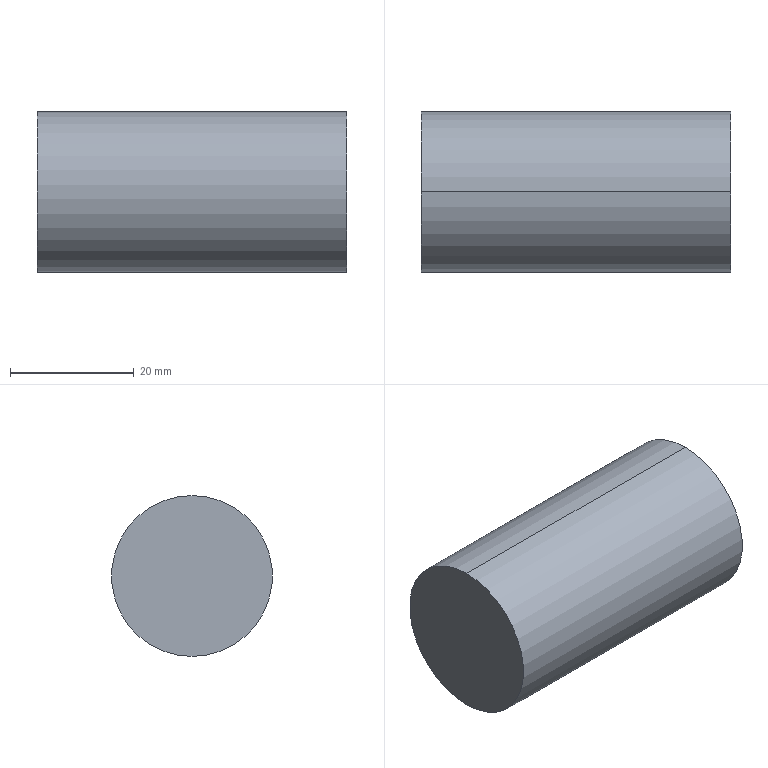Part | SolidWorks | features BaseBody 1 | 1 solid | 4 faces | box 50 x 26.001 x 26.001 mm | volume 26548 mm3 | cylinder 2 | plane 2 | commonest cylinder face diameters 26.001 x2
STEP:
#1=CARTESIAN_POINT('',(-51.,215.,-375.));
#2=VERTEX_POINT('',#1);
#3=CARTESIAN_POINT('',(-51.,215.,-401.));
#4=VERTEX_POINT('',#3);
#5=CARTESIAN_POINT('',(-51.,215.,-388.));
#6=DIRECTION('',(-1.,0.,0.));
#7=DIRECTION('',(0.,0.,1.));
#8=AXIS2_PLACEMENT_3D('',#5,#6,#7);
#9=CIRCLE('',#8,13.);
#10=EDGE_CURVE('',#2,#4,#9,.T.);
#11=ORIENTED_EDGE('',*,*,#10,.T.);
#12=CARTESIAN_POINT('',(-101.,215.,-401.));
#13=VERTEX_POINT('',#12);
#14=CARTESIAN_POINT('',(-51.,215.,-401.));
#15=DIRECTION('',(-1.,0.,0.));
#16=VECTOR('',#15,1000.);
#17=LINE('',#14,#16);
#18=EDGE_CURVE('',#4,#13,#17,.T.);
#19=ORIENTED_EDGE('',*,*,#18,.T.);
#20=CARTESIAN_POINT('',(-101.,215.,-375.));
#21=VERTEX_POINT('',#20);
#22=CARTESIAN_POINT('',(-101.,215.,-388.));
#23=DIRECTION('',(1.,0.,0.));
#24=DIRECTION('',(0.,0.,1.));
#25=AXIS2_PLACEMENT_3D('',#22,#23,#24);
#26=CIRCLE('',#25,13.);
#27=EDGE_CURVE('',#13,#21,#26,.T.);
#28=ORIENTED_EDGE('',*,*,#27,.T.);
#29=CARTESIAN_POINT('',(-51.,215.,-375.));
#30=DIRECTION('',(-1.,0.,0.));
#31=VECTOR('',#30,1000.);
#32=LINE('',#29,#31);
#33=EDGE_CURVE('',#2,#21,#32,.T.);
#34=ORIENTED_EDGE('',*,*,#33,.F.);
#35=EDGE_LOOP('',(#11,#19,#28,#34));
#36=FACE_OUTER_BOUND('',#35,.T.);
#37=CARTESIAN_POINT('',(-51.,215.,-388.));
#38=DIRECTION('',(-1.,0.,0.));
#39=DIRECTION('',(0.,0.,1.));
#40=AXIS2_PLACEMENT_3D('',#37,#38,#39);
#41=CYLINDRICAL_SURFACE('',#40,13.);
#42=ADVANCED_FACE('',(#36),#41,.T.);
#43=ORIENTED_EDGE('',*,*,#18,.F.);
#44=CARTESIAN_POINT('',(-51.,215.,-388.));
#45=DIRECTION('',(-1.,0.,0.));
#46=DIRECTION('',(0.,0.,1.));
#47=AXIS2_PLACEMENT_3D('',#44,#45,#46);
#48=CIRCLE('',#47,13.);
#49=EDGE_CURVE('',#4,#2,#48,.T.);
#50=ORIENTED_EDGE('',*,*,#49,.T.);
#51=ORIENTED_EDGE('',*,*,#33,.T.);
#52=CARTESIAN_POINT('',(-101.,215.,-388.));
#53=DIRECTION('',(1.,0.,0.));
#54=DIRECTION('',(0.,0.,1.));
#55=AXIS2_PLACEMENT_3D('',#52,#53,#54);
#56=CIRCLE('',#55,13.);
#57=EDGE_CURVE('',#21,#13,#56,.T.);
#58=ORIENTED_EDGE('',*,*,#57,.T.);
#59=EDGE_LOOP('',(#43,#50,#51,#58));
#60=FACE_OUTER_BOUND('',#59,.T.);
#61=CARTESIAN_POINT('',(-51.,215.,-388.));
#62=DIRECTION('',(-1.,0.,0.));
#63=DIRECTION('',(0.,0.,1.));
#64=AXIS2_PLACEMENT_3D('',#61,#62,#63);
#65=CYLINDRICAL_SURFACE('',#64,13.);
#66=ADVANCED_FACE('',(#60),#65,.T.);
#67=ORIENTED_EDGE('',*,*,#10,.F.);
#68=ORIENTED_EDGE('',*,*,#49,.F.);
#69=EDGE_LOOP('',(#67,#68));
#70=FACE_OUTER_BOUND('',#69,.T.);
#71=CARTESIAN_POINT('',(-51.,215.,-388.));
#72=DIRECTION('',(1.,0.,0.));
#73=DIRECTION('',(0.,0.,-1.));
#74=AXIS2_PLACEMENT_3D('',#71,#72,#73);
#75=PLANE('',#74);
#76=ADVANCED_FACE('',(#70),#75,.T.);
#77=ORIENTED_EDGE('',*,*,#57,.F.);
#78=ORIENTED_EDGE('',*,*,#27,.F.);
#79=EDGE_LOOP('',(#77,#78));
#80=FACE_OUTER_BOUND('',#79,.T.);
#81=CARTESIAN_POINT('',(-101.,215.,-388.));
#82=DIRECTION('',(1.,0.,0.));
#83=DIRECTION('',(0.,0.,-1.));
#84=AXIS2_PLACEMENT_3D('',#81,#82,#83);
#85=PLANE('',#84);
#86=ADVANCED_FACE('',(#80),#85,.F.);
#87=CLOSED_SHELL('',(#42,#66,#76,#86));
#88=MANIFOLD_SOLID_BREP('',#87);
#89=CARTESIAN_POINT('',(0.,0.,0.));
#90=DIRECTION('',(0.,0.,1.));
#91=DIRECTION('',(1.,0.,0.));
#92=AXIS2_PLACEMENT_3D('',#89,#90,#91);
#93=(LENGTH_UNIT()NAMED_UNIT(*)SI_UNIT(.MILLI.,.METRE.));
#94=UNCERTAINTY_MEASURE_WITH_UNIT(LENGTH_MEASURE(0.00001),#93,'','');
#95=(NAMED_UNIT(*)PLANE_ANGLE_UNIT()SI_UNIT($,.RADIAN.));
#96=(NAMED_UNIT(*)SI_UNIT($,.STERADIAN.)SOLID_ANGLE_UNIT());
#97=(GEOMETRIC_REPRESENTATION_CONTEXT(3)GLOBAL_UNCERTAINTY_ASSIGNED_CONTEXT((#94))GLOBAL_UNIT_ASSIGNED_CONTEXT((#93,#95,#96))REPRESENTATION_CONTEXT('',''));
#98=ADVANCED_BREP_SHAPE_REPRESENTATION('',(#88,#92),#97);